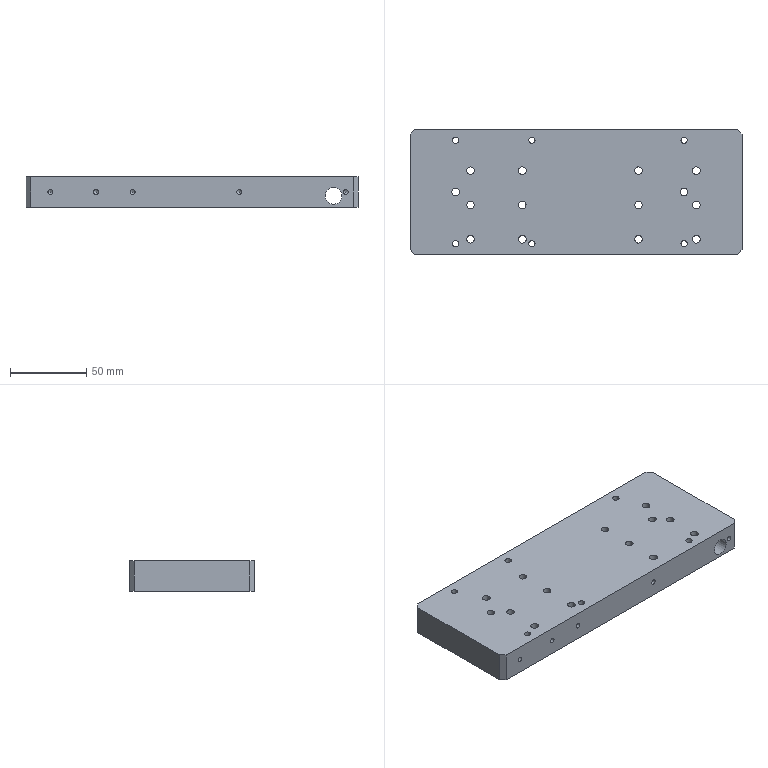CAM job | NX | 3-axis milling, drilling | part box 218 x 82 x 20 mm | stock box 223 x 87 x 25 mm
Tools:
number,name,description,diameter,corner_radius,flute_length,length,flutes
9,D10,平底铣刀-粗,10.0,0.0,35.0,75.0,2
10,D10-J,平底铣刀-精,10.0,0.0,35.0,75.0,2
1,D80R0.8飞刀,圆鼻刀-粗,80.0,0.8,50.0,75.0,2
1,D80R0.8飞刀-J,圆鼻刀-精,80.0,0.8,50.0,75.0,2
2,D6倒角刀,倒角刀,6.0,0.0,3.0,25.0,2
22,M5X0.8,丝锥,4.2,0.0,35.0,50.0,2
18,M6X1.0,丝锥,5.0,0.0,35.0,50.0,2
19,D5铰刀,Drilling Tool,5.0,0.0,75.0,100.0,6
15,ZT5.1,钻头,5.1,0.0,35.0,50.0,2
17,ZT4.9,Drilling Tool,4.9,0.0,35.0,50.0,2
14,ZT4.3,Drilling Tool,4.3,0.0,50.0,75.0,4
Operations:
program,operation,operation_type,tool,method,geometry_group,spindle_rpm,surface_speed,feed_per_tooth,feed_cut,feed_plunge,cut_length_mm,path_length_mm,cut_time_min,machine_time_min
B,底壁铣飞面开粗_COPY,VolumeBased25DMillingOperation,D80R0.8飞刀,分层开粗-切深K-步距G,W-B,2800.0,703.696,0.5357,3000.0,100.0,5802.277,6108.868,1.934,1.965
B,底壁铣飞面精光_COPY,VolumeBased25DMillingOperation,D80R0.8飞刀-J,侧刃精光-切深K-步距G,W-B,4000.0,1005.28,0.125,1000.0,100.0,644.11,740.11,0.6441,0.6537
B,NG_钻倒角_1,Operation,D6倒角刀,METHOD,W-B,8000.0,150.796,0.0625,1000.0,0.0,34.2,519.757,0.0342,0.0828
B,NG_钻倒角DJ10_1,Operation,D6倒角刀,METHOD,W-B,8000.0,150.796,0.0625,1000.0,0.0,34.8,351.703,0.0348,0.0665
B,铣倒角_4,PlanarMilling,D6倒角刀,METHOD,W-B,8000.0,150.796,0.0375,600.0,100.0,153.573,1278.455,0.256,0.3684
B,C0.3封闭铣廓倒角6X45L_COPY,PlanarMilling,D6倒角刀,爬面_倒角-切深0-步距G,W-B,7000.0,131.0,0.1071,1500.0,100.0,610.499,706.499,0.407,0.4166
A,顶面,FaceMilling,D80R0.8飞刀,侧刃精光-切深K-步距G,W-A,4500.0,1385.0,0.1667,1500.0,100.0,664.0,760.0,0.4427,0.4523
A,外形粗_2,VolumeBased25DMillingOperation,D10,METHOD,W-A,8000.0,251.327,0.375,6000.0,80.0,16876.913,16995.413,2.813,2.825
A,打点-深0.8,Operation,D6倒角刀,NONE,W-A,8000.0,150.796,0.0312,500.0,90.0,36.0,620.234,0.072,0.1304
A,通孔-M5螺纹底孔,Operation,ZT4.3,NONE,W-A,3000.0,39.584,0.0583,350.0,90.0,174.0,789.04,0.4971,0.5586
A,通孔-精孔6.0预钻,Operation,ZT4.9,NONE,W-A,2500.0,38.484,0.05,250.0,90.0,152.487,576.137,0.6099,0.6523
A,通孔-M6螺纹底孔,Operation,ZT5.1,NONE,W-A,2800.0,44.862,0.0625,350.0,90.0,228.258,873.875,0.6522,0.7167
A,仅选体,SurfaceContour,D6倒角刀,METHOD,W-A,8000.0,150.796,0.1875,3000.0,100.0,610.272,706.073,0.2034,0.213
A,铣倒角_1,PlanarMilling,D6倒角刀,METHOD,W-A,8000.0,150.796,0.0312,500.0,100.0,108.122,1050.17,0.2162,0.3104
A,铣倒角_2,PlanarMilling,D6倒角刀,METHOD,W-A,8000.0,150.796,0.0312,500.0,100.0,110.889,881.388,0.2218,0.2988
A,铣倒角_3,PlanarMilling,D6倒角刀,METHOD,W-A,8000.0,150.796,0.0312,500.0,100.0,161.526,1281.678,0.3231,0.4351
A,G85铰孔L_COPY,Operation,D5铰刀,钻孔-切深G-步距G,W-A,500.0,6.0,0.05,50.0,90.0,132.0,535.163,2.64,2.68
A,通孔-攻牙M5,Operation,M5X0.8,METHOD,W-A,500.0,6.597,0.0008,0.8,90.0,147.0,735.04,183.75,183.809
A,通孔-攻牙M6,Operation,M6X1.0,METHOD,W-A,500.0,7.854,0.001,1.0,90.0,196.0,809.36,196.0,196.061
A,外形半精_2,VolumeBased25DMillingOperation,D10-J,METHOD,W-A,9000.0,169.646,0.0667,1200.0,100.0,1258.689,1519.204,1.049,1.075